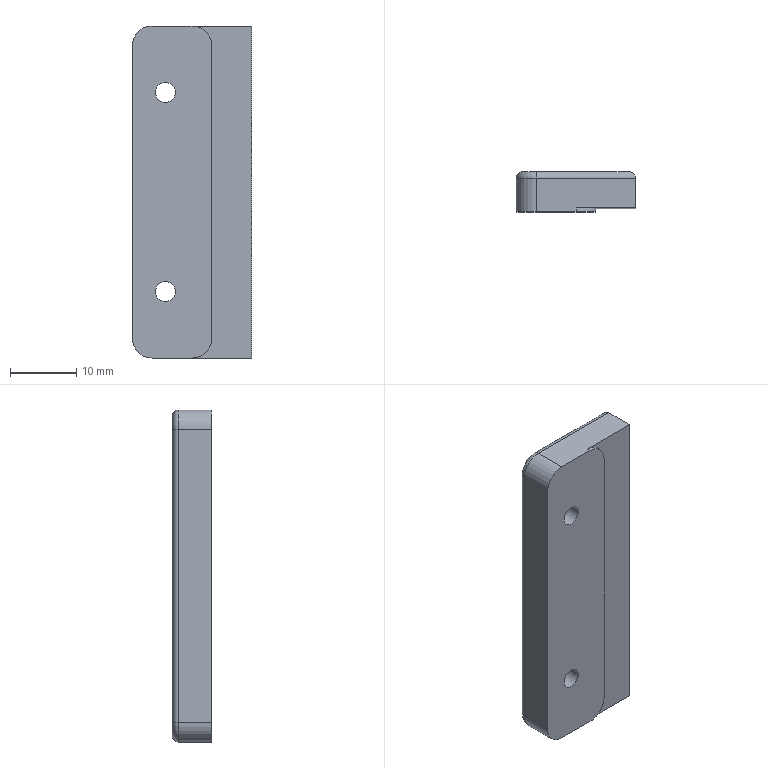Part | SolidWorks | features Fillet 4, ICE 3, Extrusion 1 | 1 solid | 28 faces | box 18 x 6 x 50 mm | volume 5021 mm3 | cylinder 16 | plane 10 | torus 2 | commonest cylinder face diameters 2 x4 3 x4 5 x4 6 x4
STEP:
#1=CARTESIAN_POINT('',(1.763,0.,10.));
#2=VERTEX_POINT('',#1);
#3=CARTESIAN_POINT('',(-1.237,0.,10.));
#4=VERTEX_POINT('',#3);
#5=CARTESIAN_POINT('',(0.2632,0.,10.));
#6=DIRECTION('',(0.,1.,0.));
#7=DIRECTION('',(-1.,0.,0.));
#8=AXIS2_PLACEMENT_3D('',#5,#6,#7);
#9=CIRCLE('',#8,1.5);
#10=EDGE_CURVE('',#2,#4,#9,.T.);
#11=ORIENTED_EDGE('',*,*,#10,.F.);
#12=CARTESIAN_POINT('',(1.763,3.,10.));
#13=VERTEX_POINT('',#12);
#14=CARTESIAN_POINT('',(1.763,0.,10.));
#15=DIRECTION('',(0.,1.,0.));
#16=VECTOR('',#15,1000.);
#17=LINE('',#14,#16);
#18=EDGE_CURVE('',#2,#13,#17,.T.);
#19=ORIENTED_EDGE('',*,*,#18,.T.);
#20=CARTESIAN_POINT('',(-1.237,3.,10.));
#21=VERTEX_POINT('',#20);
#22=CARTESIAN_POINT('',(0.2632,3.,10.));
#23=DIRECTION('',(0.,1.,0.));
#24=DIRECTION('',(-1.,0.,0.));
#25=AXIS2_PLACEMENT_3D('',#22,#23,#24);
#26=CIRCLE('',#25,1.5);
#27=EDGE_CURVE('',#13,#21,#26,.T.);
#28=ORIENTED_EDGE('',*,*,#27,.T.);
#29=CARTESIAN_POINT('',(-1.237,0.,10.));
#30=DIRECTION('',(0.,1.,0.));
#31=VECTOR('',#30,1000.);
#32=LINE('',#29,#31);
#33=EDGE_CURVE('',#4,#21,#32,.T.);
#34=ORIENTED_EDGE('',*,*,#33,.F.);
#35=EDGE_LOOP('',(#11,#19,#28,#34));
#36=FACE_OUTER_BOUND('',#35,.T.);
#37=CARTESIAN_POINT('',(0.2632,0.,10.));
#38=DIRECTION('',(0.,1.,0.));
#39=DIRECTION('',(-1.,0.,0.));
#40=AXIS2_PLACEMENT_3D('',#37,#38,#39);
#41=CYLINDRICAL_SURFACE('',#40,1.5);
#42=ADVANCED_FACE('',(#36),#41,.F.);
#43=CARTESIAN_POINT('',(1.763,0.,40.));
#44=VERTEX_POINT('',#43);
#45=CARTESIAN_POINT('',(-1.237,0.,40.));
#46=VERTEX_POINT('',#45);
#47=CARTESIAN_POINT('',(0.2632,0.,40.));
#48=DIRECTION('',(0.,1.,0.));
#49=DIRECTION('',(-1.,0.,0.));
#50=AXIS2_PLACEMENT_3D('',#47,#48,#49);
#51=CIRCLE('',#50,1.5);
#52=EDGE_CURVE('',#44,#46,#51,.T.);
#53=ORIENTED_EDGE('',*,*,#52,.F.);
#54=CARTESIAN_POINT('',(1.763,3.,40.));
#55=VERTEX_POINT('',#54);
#56=CARTESIAN_POINT('',(1.763,0.,40.));
#57=DIRECTION('',(0.,1.,0.));
#58=VECTOR('',#57,1000.);
#59=LINE('',#56,#58);
#60=EDGE_CURVE('',#44,#55,#59,.T.);
#61=ORIENTED_EDGE('',*,*,#60,.T.);
#62=CARTESIAN_POINT('',(-1.237,3.,40.));
#63=VERTEX_POINT('',#62);
#64=CARTESIAN_POINT('',(0.2632,3.,40.));
#65=DIRECTION('',(0.,1.,0.));
#66=DIRECTION('',(-1.,0.,0.));
#67=AXIS2_PLACEMENT_3D('',#64,#65,#66);
#68=CIRCLE('',#67,1.5);
#69=EDGE_CURVE('',#55,#63,#68,.T.);
#70=ORIENTED_EDGE('',*,*,#69,.T.);
#71=CARTESIAN_POINT('',(-1.237,0.,40.));
#72=DIRECTION('',(0.,1.,0.));
#73=VECTOR('',#72,1000.);
#74=LINE('',#71,#73);
#75=EDGE_CURVE('',#46,#63,#74,.T.);
#76=ORIENTED_EDGE('',*,*,#75,.F.);
#77=EDGE_LOOP('',(#53,#61,#70,#76));
#78=FACE_OUTER_BOUND('',#77,.T.);
#79=CARTESIAN_POINT('',(0.2632,0.,40.));
#80=DIRECTION('',(0.,1.,0.));
#81=DIRECTION('',(-1.,0.,0.));
#82=AXIS2_PLACEMENT_3D('',#79,#80,#81);
#83=CYLINDRICAL_SURFACE('',#82,1.5);
#84=ADVANCED_FACE('',(#78),#83,.F.);
#85=CARTESIAN_POINT('',(2.763,3.,10.));
#86=VERTEX_POINT('',#85);
#87=CARTESIAN_POINT('',(-2.237,3.,10.));
#88=VERTEX_POINT('',#87);
#89=CARTESIAN_POINT('',(0.2632,3.,10.));
#90=DIRECTION('',(0.,1.,0.));
#91=DIRECTION('',(-1.,0.,0.));
#92=AXIS2_PLACEMENT_3D('',#89,#90,#91);
#93=CIRCLE('',#92,2.5);
#94=EDGE_CURVE('',#86,#88,#93,.T.);
#95=ORIENTED_EDGE('',*,*,#94,.F.);
#96=CARTESIAN_POINT('',(2.763,6.,10.));
#97=VERTEX_POINT('',#96);
#98=CARTESIAN_POINT('',(2.763,3.,10.));
#99=DIRECTION('',(0.,1.,0.));
#100=VECTOR('',#99,1000.);
#101=LINE('',#98,#100);
#102=EDGE_CURVE('',#86,#97,#101,.T.);
#103=ORIENTED_EDGE('',*,*,#102,.T.);
#104=CARTESIAN_POINT('',(-2.237,6.,10.));
#105=VERTEX_POINT('',#104);
#106=CARTESIAN_POINT('',(0.2632,6.,10.));
#107=DIRECTION('',(0.,1.,0.));
#108=DIRECTION('',(-1.,0.,0.));
#109=AXIS2_PLACEMENT_3D('',#106,#107,#108);
#110=CIRCLE('',#109,2.5);
#111=EDGE_CURVE('',#97,#105,#110,.T.);
#112=ORIENTED_EDGE('',*,*,#111,.T.);
#113=CARTESIAN_POINT('',(-2.237,3.,10.));
#114=DIRECTION('',(0.,1.,0.));
#115=VECTOR('',#114,1000.);
#116=LINE('',#113,#115);
#117=EDGE_CURVE('',#88,#105,#116,.T.);
#118=ORIENTED_EDGE('',*,*,#117,.F.);
#119=EDGE_LOOP('',(#95,#103,#112,#118));
#120=FACE_OUTER_BOUND('',#119,.T.);
#121=CARTESIAN_POINT('',(0.2632,3.,10.));
#122=DIRECTION('',(0.,1.,0.));
#123=DIRECTION('',(-1.,0.,0.));
#124=AXIS2_PLACEMENT_3D('',#121,#122,#123);
#125=CYLINDRICAL_SURFACE('',#124,2.5);
#126=ADVANCED_FACE('',(#120),#125,.F.);
#127=CARTESIAN_POINT('',(2.763,3.,40.));
#128=VERTEX_POINT('',#127);
#129=CARTESIAN_POINT('',(-2.237,3.,40.));
#130=VERTEX_POINT('',#129);
#131=CARTESIAN_POINT('',(0.2632,3.,40.));
#132=DIRECTION('',(0.,1.,0.));
#133=DIRECTION('',(-1.,0.,0.));
#134=AXIS2_PLACEMENT_3D('',#131,#132,#133);
#135=CIRCLE('',#134,2.5);
#136=EDGE_CURVE('',#128,#130,#135,.T.);
#137=ORIENTED_EDGE('',*,*,#136,.F.);
#138=CARTESIAN_POINT('',(2.763,6.,40.));
#139=VERTEX_POINT('',#138);
#140=CARTESIAN_POINT('',(2.763,3.,40.));
#141=DIRECTION('',(0.,1.,0.));
#142=VECTOR('',#141,1000.);
#143=LINE('',#140,#142);
#144=EDGE_CURVE('',#128,#139,#143,.T.);
#145=ORIENTED_EDGE('',*,*,#144,.T.);
#146=CARTESIAN_POINT('',(-2.237,6.,40.));
#147=VERTEX_POINT('',#146);
#148=CARTESIAN_POINT('',(0.2632,6.,40.));
#149=DIRECTION('',(0.,1.,0.));
#150=DIRECTION('',(-1.,0.,0.));
#151=AXIS2_PLACEMENT_3D('',#148,#149,#150);
#152=CIRCLE('',#151,2.5);
#153=EDGE_CURVE('',#139,#147,#152,.T.);
#154=ORIENTED_EDGE('',*,*,#153,.T.);
#155=CARTESIAN_POINT('',(-2.237,3.,40.));
#156=DIRECTION('',(0.,1.,0.));
#157=VECTOR('',#156,1000.);
#158=LINE('',#155,#157);
#159=EDGE_CURVE('',#130,#147,#158,.T.);
#160=ORIENTED_EDGE('',*,*,#159,.F.);
#161=EDGE_LOOP('',(#137,#145,#154,#160));
#162=FACE_OUTER_BOUND('',#161,.T.);
#163=CARTESIAN_POINT('',(0.2632,3.,40.));
#164=DIRECTION('',(0.,1.,0.));
#165=DIRECTION('',(-1.,0.,0.));
#166=AXIS2_PLACEMENT_3D('',#163,#164,#165);
#167=CYLINDRICAL_SURFACE('',#166,2.5);
#168=ADVANCED_FACE('',(#162),#167,.F.);
#169=CARTESIAN_POINT('',(0.2632,0.,10.));
#170=DIRECTION('',(0.,1.,0.));
#171=DIRECTION('',(-1.,0.,0.));
#172=AXIS2_PLACEMENT_3D('',#169,#170,#171);
#173=CIRCLE('',#172,1.5);
#174=EDGE_CURVE('',#4,#2,#173,.T.);
#175=ORIENTED_EDGE('',*,*,#174,.T.);
#176=ORIENTED_EDGE('',*,*,#10,.T.);
#177=EDGE_LOOP('',(#175,#176));
#178=FACE_BOUND('',#177,.T.);
#179=CARTESIAN_POINT('',(0.2632,0.,40.));
#180=DIRECTION('',(0.,1.,0.));
#181=DIRECTION('',(-1.,0.,0.));
#182=AXIS2_PLACEMENT_3D('',#179,#180,#181);
#183=CIRCLE('',#182,1.5);
#184=EDGE_CURVE('',#46,#44,#183,.T.);
#185=ORIENTED_EDGE('',*,*,#184,.T.);
#186=ORIENTED_EDGE('',*,*,#52,.T.);
#187=EDGE_LOOP('',(#185,#186));
#188=FACE_BOUND('',#187,.T.);
#189=CARTESIAN_POINT('',(-4.737,0.,47.));
#190=VERTEX_POINT('',#189);
#191=CARTESIAN_POINT('',(-4.737,0.,3.));
#192=VERTEX_POINT('',#191);
#193=CARTESIAN_POINT('',(-4.737,0.,50.));
#194=DIRECTION('',(0.,0.,-1.));
#195=VECTOR('',#194,1000.);
#196=LINE('',#193,#195);
#197=EDGE_CURVE('',#190,#192,#196,.T.);
#198=ORIENTED_EDGE('',*,*,#197,.T.);
#199=CARTESIAN_POINT('',(-1.737,0.,0.));
#200=VERTEX_POINT('',#199);
#201=CARTESIAN_POINT('',(-1.737,0.,3.));
#202=DIRECTION('',(0.,-1.,0.));
#203=DIRECTION('',(-1.,0.,0.));
#204=AXIS2_PLACEMENT_3D('',#201,#202,#203);
#205=CIRCLE('',#204,3.);
#206=EDGE_CURVE('',#192,#200,#205,.T.);
#207=ORIENTED_EDGE('',*,*,#206,.T.);
#208=CARTESIAN_POINT('',(4.263,0.,0.));
#209=VERTEX_POINT('',#208);
#210=CARTESIAN_POINT('',(7.263,0.,0.));
#211=DIRECTION('',(1.,0.,0.));
#212=VECTOR('',#211,1000.);
#213=LINE('',#210,#212);
#214=EDGE_CURVE('',#200,#209,#213,.T.);
#215=ORIENTED_EDGE('',*,*,#214,.T.);
#216=CARTESIAN_POINT('',(7.263,0.,3.));
#217=VERTEX_POINT('',#216);
#218=CARTESIAN_POINT('',(4.263,0.,3.));
#219=DIRECTION('',(0.,-1.,0.));
#220=DIRECTION('',(-1.,0.,0.));
#221=AXIS2_PLACEMENT_3D('',#218,#219,#220);
#222=CIRCLE('',#221,3.);
#223=EDGE_CURVE('',#209,#217,#222,.T.);
#224=ORIENTED_EDGE('',*,*,#223,.T.);
#225=CARTESIAN_POINT('',(7.263,0.,47.));
#226=VERTEX_POINT('',#225);
#227=CARTESIAN_POINT('',(7.263,0.,50.));
#228=DIRECTION('',(0.,0.,-1.));
#229=VECTOR('',#228,1000.);
#230=LINE('',#227,#229);
#231=EDGE_CURVE('',#226,#217,#230,.T.);
#232=ORIENTED_EDGE('',*,*,#231,.F.);
#233=CARTESIAN_POINT('',(4.263,0.,50.));
#234=VERTEX_POINT('',#233);
#235=CARTESIAN_POINT('',(4.263,0.,47.));
#236=DIRECTION('',(0.,-1.,0.));
#237=DIRECTION('',(-1.,0.,0.));
#238=AXIS2_PLACEMENT_3D('',#235,#236,#237);
#239=CIRCLE('',#238,3.);
#240=EDGE_CURVE('',#226,#234,#239,.T.);
#241=ORIENTED_EDGE('',*,*,#240,.T.);
#242=CARTESIAN_POINT('',(-1.737,0.,50.));
#243=VERTEX_POINT('',#242);
#244=CARTESIAN_POINT('',(7.263,0.,50.));
#245=DIRECTION('',(1.,0.,0.));
#246=VECTOR('',#245,1000.);
#247=LINE('',#244,#246);
#248=EDGE_CURVE('',#243,#234,#247,.T.);
#249=ORIENTED_EDGE('',*,*,#248,.F.);
#250=CARTESIAN_POINT('',(-1.737,0.,47.));
#251=DIRECTION('',(0.,-1.,0.));
#252=DIRECTION('',(-1.,0.,0.));
#253=AXIS2_PLACEMENT_3D('',#250,#251,#252);
#254=CIRCLE('',#253,3.);
#255=EDGE_CURVE('',#243,#190,#254,.T.);
#256=ORIENTED_EDGE('',*,*,#255,.T.);
#257=EDGE_LOOP('',(#198,#207,#215,#224,#232,#241,#249,#256));
#258=FACE_OUTER_BOUND('',#257,.T.);
#259=CARTESIAN_POINT('',(7.263,0.,50.));
#260=DIRECTION('',(0.,1.,0.));
#261=DIRECTION('',(-1.,0.,0.));
#262=AXIS2_PLACEMENT_3D('',#259,#260,#261);
#263=PLANE('',#262);
#264=ADVANCED_FACE('',(#178,#188,#258),#263,.F.);
#265=ORIENTED_EDGE('',*,*,#231,.T.);
#266=CARTESIAN_POINT('',(7.263,0.55,3.));
#267=VERTEX_POINT('',#266);
#268=CARTESIAN_POINT('',(7.263,0.55,3.));
#269=DIRECTION('',(0.,1.,0.));
#270=VECTOR('',#269,1000.);
#271=LINE('',#268,#270);
#272=EDGE_CURVE('',#217,#267,#271,.T.);
#273=ORIENTED_EDGE('',*,*,#272,.T.);
#274=CARTESIAN_POINT('',(7.263,0.55,47.));
#275=VERTEX_POINT('',#274);
#276=CARTESIAN_POINT('',(7.263,0.55,50.));
#277=DIRECTION('',(0.,0.,-1.));
#278=VECTOR('',#277,1000.);
#279=LINE('',#276,#278);
#280=EDGE_CURVE('',#275,#267,#279,.T.);
#281=ORIENTED_EDGE('',*,*,#280,.F.);
#282=CARTESIAN_POINT('',(7.263,0.55,47.));
#283=DIRECTION('',(0.,-1.,0.));
#284=VECTOR('',#283,1000.);
#285=LINE('',#282,#284);
#286=EDGE_CURVE('',#275,#226,#285,.T.);
#287=ORIENTED_EDGE('',*,*,#286,.T.);
#288=EDGE_LOOP('',(#265,#273,#281,#287));
#289=FACE_OUTER_BOUND('',#288,.T.);
#290=CARTESIAN_POINT('',(7.263,0.55,50.));
#291=DIRECTION('',(-1.,0.,0.));
#292=DIRECTION('',(0.,-1.,0.));
#293=AXIS2_PLACEMENT_3D('',#290,#291,#292);
#294=PLANE('',#293);
#295=ADVANCED_FACE('',(#289),#294,.F.);
#296=CARTESIAN_POINT('',(4.263,0.55,0.));
#297=VERTEX_POINT('',#296);
#298=CARTESIAN_POINT('',(13.263,0.55,0.));
#299=VERTEX_POINT('',#298);
#300=CARTESIAN_POINT('',(13.263,0.55,0.));
#301=DIRECTION('',(1.,0.,0.));
#302=VECTOR('',#301,1000.);
#303=LINE('',#300,#302);
#304=EDGE_CURVE('',#297,#299,#303,.T.);
#305=ORIENTED_EDGE('',*,*,#304,.T.);
#306=CARTESIAN_POINT('',(13.263,0.55,50.));
#307=VERTEX_POINT('',#306);
#308=CARTESIAN_POINT('',(13.263,0.55,50.));
#309=DIRECTION('',(0.,0.,-1.));
#310=VECTOR('',#309,1000.);
#311=LINE('',#308,#310);
#312=EDGE_CURVE('',#307,#299,#311,.T.);
#313=ORIENTED_EDGE('',*,*,#312,.F.);
#314=CARTESIAN_POINT('',(4.263,0.55,50.));
#315=VERTEX_POINT('',#314);
#316=CARTESIAN_POINT('',(13.263,0.55,50.));
#317=DIRECTION('',(1.,0.,0.));
#318=VECTOR('',#317,1000.);
#319=LINE('',#316,#318);
#320=EDGE_CURVE('',#315,#307,#319,.T.);
#321=ORIENTED_EDGE('',*,*,#320,.F.);
#322=CARTESIAN_POINT('',(4.263,0.55,47.));
#323=DIRECTION('',(0.,1.,0.));
#324=DIRECTION('',(-1.,0.,0.));
#325=AXIS2_PLACEMENT_3D('',#322,#323,#324);
#326=CIRCLE('',#325,3.);
#327=EDGE_CURVE('',#315,#275,#326,.T.);
#328=ORIENTED_EDGE('',*,*,#327,.T.);
#329=ORIENTED_EDGE('',*,*,#280,.T.);
#330=CARTESIAN_POINT('',(4.263,0.55,3.));
#331=DIRECTION('',(0.,1.,0.));
#332=DIRECTION('',(-1.,0.,0.));
#333=AXIS2_PLACEMENT_3D('',#330,#331,#332);
#334=CIRCLE('',#333,3.);
#335=EDGE_CURVE('',#267,#297,#334,.T.);
#336=ORIENTED_EDGE('',*,*,#335,.T.);
#337=EDGE_LOOP('',(#305,#313,#321,#328,#329,#336));
#338=FACE_OUTER_BOUND('',#337,.T.);
#339=CARTESIAN_POINT('',(13.263,0.55,50.));
#340=DIRECTION('',(0.,1.,0.));
#341=DIRECTION('',(-1.,0.,0.));
#342=AXIS2_PLACEMENT_3D('',#339,#340,#341);
#343=PLANE('',#342);
#344=ADVANCED_FACE('',(#338),#343,.F.);
#345=CARTESIAN_POINT('',(13.263,5.,0.));
#346=VERTEX_POINT('',#345);
#347=CARTESIAN_POINT('',(13.263,6.,0.));
#348=DIRECTION('',(0.,1.,0.));
#349=VECTOR('',#348,1000.);
#350=LINE('',#347,#349);
#351=EDGE_CURVE('',#299,#346,#350,.T.);
#352=ORIENTED_EDGE('',*,*,#351,.T.);
#353=CARTESIAN_POINT('',(13.263,5.,50.));
#354=VERTEX_POINT('',#353);
#355=CARTESIAN_POINT('',(13.263,5.,50.));
#356=DIRECTION('',(0.,0.,1.));
#357=VECTOR('',#356,1000.);
#358=LINE('',#355,#357);
#359=EDGE_CURVE('',#346,#354,#358,.T.);
#360=ORIENTED_EDGE('',*,*,#359,.T.);
#361=CARTESIAN_POINT('',(13.263,6.,50.));
#362=DIRECTION('',(0.,1.,0.));
#363=VECTOR('',#362,1000.);
#364=LINE('',#361,#363);
#365=EDGE_CURVE('',#307,#354,#364,.T.);
#366=ORIENTED_EDGE('',*,*,#365,.F.);
#367=ORIENTED_EDGE('',*,*,#312,.T.);
#368=EDGE_LOOP('',(#352,#360,#366,#367));
#369=FACE_OUTER_BOUND('',#368,.T.);
#370=CARTESIAN_POINT('',(13.263,6.,50.));
#371=DIRECTION('',(-1.,0.,0.));
#372=DIRECTION('',(0.,0.,1.));
#373=AXIS2_PLACEMENT_3D('',#370,#371,#372);
#374=PLANE('',#373);
#375=ADVANCED_FACE('',(#369),#374,.F.);
#376=CARTESIAN_POINT('',(-3.737,6.,47.));
#377=VERTEX_POINT('',#376);
#378=CARTESIAN_POINT('',(-1.737,6.,49.));
#379=VERTEX_POINT('',#378);
#380=CARTESIAN_POINT('',(-1.737,6.,47.));
#381=DIRECTION('',(0.,1.,0.));
#382=DIRECTION('',(0.,0.,-1.));
#383=AXIS2_PLACEMENT_3D('',#380,#381,#382);
#384=CIRCLE('',#383,2.);
#385=EDGE_CURVE('',#377,#379,#384,.T.);
#386=ORIENTED_EDGE('',*,*,#385,.T.);
#387=CARTESIAN_POINT('',(12.263,6.,49.));
#388=VERTEX_POINT('',#387);
#389=CARTESIAN_POINT('',(-4.737,6.,49.));
#390=DIRECTION('',(1.,0.,0.));
#391=VECTOR('',#390,1000.);
#392=LINE('',#389,#391);
#393=EDGE_CURVE('',#379,#388,#392,.T.);
#394=ORIENTED_EDGE('',*,*,#393,.T.);
#395=CARTESIAN_POINT('',(12.263,6.,1.));
#396=VERTEX_POINT('',#395);
#397=CARTESIAN_POINT('',(12.263,6.,50.));
#398=DIRECTION('',(0.,0.,-1.));
#399=VECTOR('',#398,1000.);
#400=LINE('',#397,#399);
#401=EDGE_CURVE('',#388,#396,#400,.T.);
#402=ORIENTED_EDGE('',*,*,#401,.T.);
#403=CARTESIAN_POINT('',(-1.737,6.,1.));
#404=VERTEX_POINT('',#403);
#405=CARTESIAN_POINT('',(-1.737,6.,1.));
#406=DIRECTION('',(-1.,0.,0.));
#407=VECTOR('',#406,1000.);
#408=LINE('',#405,#407);
#409=EDGE_CURVE('',#396,#404,#408,.T.);
#410=ORIENTED_EDGE('',*,*,#409,.T.);
#411=CARTESIAN_POINT('',(-3.737,6.,3.));
#412=VERTEX_POINT('',#411);
#413=CARTESIAN_POINT('',(-1.737,6.,3.));
#414=DIRECTION('',(0.,1.,0.));
#415=DIRECTION('',(0.,0.,-1.));
#416=AXIS2_PLACEMENT_3D('',#413,#414,#415);
#417=CIRCLE('',#416,2.);
#418=EDGE_CURVE('',#404,#412,#417,.T.);
#419=ORIENTED_EDGE('',*,*,#418,.T.);
#420=CARTESIAN_POINT('',(-3.737,6.,50.));
#421=DIRECTION('',(0.,0.,1.));
#422=VECTOR('',#421,1000.);
#423=LINE('',#420,#422);
#424=EDGE_CURVE('',#412,#377,#423,.T.);
#425=ORIENTED_EDGE('',*,*,#424,.T.);
#426=EDGE_LOOP('',(#386,#394,#402,#410,#419,#425));
#427=FACE_OUTER_BOUND('',#426,.T.);
#428=CARTESIAN_POINT('',(0.2632,6.,10.));
#429=DIRECTION('',(0.,1.,0.));
#430=DIRECTION('',(-1.,0.,0.));
#431=AXIS2_PLACEMENT_3D('',#428,#429,#430);
#432=CIRCLE('',#431,2.5);
#433=EDGE_CURVE('',#105,#97,#432,.T.);
#434=ORIENTED_EDGE('',*,*,#433,.F.);
#435=ORIENTED_EDGE('',*,*,#111,.F.);
#436=EDGE_LOOP('',(#434,#435));
#437=FACE_BOUND('',#436,.T.);
#438=CARTESIAN_POINT('',(0.2632,6.,40.));
#439=DIRECTION('',(0.,1.,0.));
#440=DIRECTION('',(-1.,0.,0.));
#441=AXIS2_PLACEMENT_3D('',#438,#439,#440);
#442=CIRCLE('',#441,2.5);
#443=EDGE_CURVE('',#147,#139,#442,.T.);
#444=ORIENTED_EDGE('',*,*,#443,.F.);
#445=ORIENTED_EDGE('',*,*,#153,.F.);
#446=EDGE_LOOP('',(#444,#445));
#447=FACE_BOUND('',#446,.T.);
#448=CARTESIAN_POINT('',(-4.737,6.,50.));
#449=DIRECTION('',(0.,-1.,0.));
#450=DIRECTION('',(0.,0.,-1.));
#451=AXIS2_PLACEMENT_3D('',#448,#449,#450);
#452=PLANE('',#451);
#453=ADVANCED_FACE('',(#427,#437,#447),#452,.F.);
#454=CARTESIAN_POINT('',(-4.737,5.,47.));
#455=VERTEX_POINT('',#454);
#456=CARTESIAN_POINT('',(-4.737,0.,47.));
#457=DIRECTION('',(0.,1.,0.));
#458=VECTOR('',#457,1000.);
#459=LINE('',#456,#458);
#460=EDGE_CURVE('',#190,#455,#459,.T.);
#461=ORIENTED_EDGE('',*,*,#460,.T.);
#462=CARTESIAN_POINT('',(-4.737,5.,3.));
#463=VERTEX_POINT('',#462);
#464=CARTESIAN_POINT('',(-4.737,5.,50.));
#465=DIRECTION('',(0.,0.,-1.));
#466=VECTOR('',#465,1000.);
#467=LINE('',#464,#466);
#468=EDGE_CURVE('',#455,#463,#467,.T.);
#469=ORIENTED_EDGE('',*,*,#468,.T.);
#470=CARTESIAN_POINT('',(-4.737,0.,3.));
#471=DIRECTION('',(0.,-1.,0.));
#472=VECTOR('',#471,1000.);
#473=LINE('',#470,#472);
#474=EDGE_CURVE('',#463,#192,#473,.T.);
#475=ORIENTED_EDGE('',*,*,#474,.T.);
#476=ORIENTED_EDGE('',*,*,#197,.F.);
#477=EDGE_LOOP('',(#461,#469,#475,#476));
#478=FACE_OUTER_BOUND('',#477,.T.);
#479=CARTESIAN_POINT('',(-4.737,0.,50.));
#480=DIRECTION('',(1.,0.,0.));
#481=DIRECTION('',(0.,0.,-1.));
#482=AXIS2_PLACEMENT_3D('',#479,#480,#481);
#483=PLANE('',#482);
#484=ADVANCED_FACE('',(#478),#483,.F.);
#485=ORIENTED_EDGE('',*,*,#365,.T.);
#486=CARTESIAN_POINT('',(-1.737,5.,50.));
#487=VERTEX_POINT('',#486);
#488=CARTESIAN_POINT('',(0.,5.,50.));
#489=DIRECTION('',(-1.,0.,0.));
#490=VECTOR('',#489,1000.);
#491=LINE('',#488,#490);
#492=EDGE_CURVE('',#354,#487,#491,.T.);
#493=ORIENTED_EDGE('',*,*,#492,.T.);
#494=CARTESIAN_POINT('',(-1.737,0.,50.));
#495=DIRECTION('',(0.,-1.,0.));
#496=VECTOR('',#495,1000.);
#497=LINE('',#494,#496);
#498=EDGE_CURVE('',#487,#243,#497,.T.);
#499=ORIENTED_EDGE('',*,*,#498,.T.);
#500=ORIENTED_EDGE('',*,*,#248,.T.);
#501=CARTESIAN_POINT('',(4.263,0.,50.));
#502=DIRECTION('',(0.,1.,0.));
#503=VECTOR('',#502,1000.);
#504=LINE('',#501,#503);
#505=EDGE_CURVE('',#234,#315,#504,.T.);
#506=ORIENTED_EDGE('',*,*,#505,.T.);
#507=ORIENTED_EDGE('',*,*,#320,.T.);
#508=EDGE_LOOP('',(#485,#493,#499,#500,#506,#507));
#509=FACE_OUTER_BOUND('',#508,.T.);
#510=CARTESIAN_POINT('',(0.,0.,50.));
#511=DIRECTION('',(0.,0.,-1.));
#512=DIRECTION('',(-1.,0.,0.));
#513=AXIS2_PLACEMENT_3D('',#510,#511,#512);
#514=PLANE('',#513);
#515=ADVANCED_FACE('',(#509),#514,.F.);
#516=CARTESIAN_POINT('',(-1.737,5.,0.));
#517=VERTEX_POINT('',#516);
#518=CARTESIAN_POINT('',(-1.737,6.,0.));
#519=DIRECTION('',(0.,1.,0.));
#520=VECTOR('',#519,1000.);
#521=LINE('',#518,#520);
#522=EDGE_CURVE('',#200,#517,#521,.T.);
#523=ORIENTED_EDGE('',*,*,#522,.T.);
#524=CARTESIAN_POINT('',(13.263,5.,0.));
#525=DIRECTION('',(1.,0.,0.));
#526=VECTOR('',#525,1000.);
#527=LINE('',#524,#526);
#528=EDGE_CURVE('',#517,#346,#527,.T.);
#529=ORIENTED_EDGE('',*,*,#528,.T.);
#530=ORIENTED_EDGE('',*,*,#351,.F.);
#531=ORIENTED_EDGE('',*,*,#304,.F.);
#532=CARTESIAN_POINT('',(4.263,0.,0.));
#533=DIRECTION('',(0.,-1.,0.));
#534=VECTOR('',#533,1000.);
#535=LINE('',#532,#534);
#536=EDGE_CURVE('',#297,#209,#535,.T.);
#537=ORIENTED_EDGE('',*,*,#536,.T.);
#538=ORIENTED_EDGE('',*,*,#214,.F.);
#539=EDGE_LOOP('',(#523,#529,#530,#531,#537,#538));
#540=FACE_OUTER_BOUND('',#539,.T.);
#541=CARTESIAN_POINT('',(0.,0.,0.));
#542=DIRECTION('',(0.,0.,-1.));
#543=DIRECTION('',(-1.,0.,0.));
#544=AXIS2_PLACEMENT_3D('',#541,#542,#543);
#545=PLANE('',#544);
#546=ADVANCED_FACE('',(#540),#545,.T.);
#547=ORIENTED_EDGE('',*,*,#240,.F.);
#548=ORIENTED_EDGE('',*,*,#286,.F.);
#549=ORIENTED_EDGE('',*,*,#327,.F.);
#550=ORIENTED_EDGE('',*,*,#505,.F.);
#551=EDGE_LOOP('',(#547,#548,#549,#550));
#552=FACE_OUTER_BOUND('',#551,.T.);
#553=CARTESIAN_POINT('',(4.263,0.,47.));
#554=DIRECTION('',(0.,1.,0.));
#555=DIRECTION('',(-1.,0.,0.));
#556=AXIS2_PLACEMENT_3D('',#553,#554,#555);
#557=CYLINDRICAL_SURFACE('',#556,3.);
#558=ADVANCED_FACE('',(#552),#557,.T.);
#559=ORIENTED_EDGE('',*,*,#144,.F.);
#560=CARTESIAN_POINT('',(0.2632,3.,40.));
#561=DIRECTION('',(0.,1.,0.));
#562=DIRECTION('',(-1.,0.,0.));
#563=AXIS2_PLACEMENT_3D('',#560,#561,#562);
#564=CIRCLE('',#563,2.5);
#565=EDGE_CURVE('',#130,#128,#564,.T.);
#566=ORIENTED_EDGE('',*,*,#565,.F.);
#567=ORIENTED_EDGE('',*,*,#159,.T.);
#568=ORIENTED_EDGE('',*,*,#443,.T.);
#569=EDGE_LOOP('',(#559,#566,#567,#568));
#570=FACE_OUTER_BOUND('',#569,.T.);
#571=CARTESIAN_POINT('',(0.2632,3.,40.));
#572=DIRECTION('',(0.,1.,0.));
#573=DIRECTION('',(-1.,0.,0.));
#574=AXIS2_PLACEMENT_3D('',#571,#572,#573);
#575=CYLINDRICAL_SURFACE('',#574,2.5);
#576=ADVANCED_FACE('',(#570),#575,.F.);
#577=CARTESIAN_POINT('',(0.2632,3.,40.));
#578=DIRECTION('',(0.,1.,0.));
#579=DIRECTION('',(-1.,0.,0.));
#580=AXIS2_PLACEMENT_3D('',#577,#578,#579);
#581=CIRCLE('',#580,1.5);
#582=EDGE_CURVE('',#63,#55,#581,.T.);
#583=ORIENTED_EDGE('',*,*,#582,.F.);
#584=ORIENTED_EDGE('',*,*,#69,.F.);
#585=EDGE_LOOP('',(#583,#584));
#586=FACE_BOUND('',#585,.T.);
#587=ORIENTED_EDGE('',*,*,#565,.T.);
#588=ORIENTED_EDGE('',*,*,#136,.T.);
#589=EDGE_LOOP('',(#587,#588));
#590=FACE_OUTER_BOUND('',#589,.T.);
#591=CARTESIAN_POINT('',(0.2632,3.,40.));
#592=DIRECTION('',(0.,1.,0.));
#593=DIRECTION('',(-1.,0.,0.));
#594=AXIS2_PLACEMENT_3D('',#591,#592,#593);
#595=PLANE('',#594);
#596=ADVANCED_FACE('',(#586,#590),#595,.T.);
#597=ORIENTED_EDGE('',*,*,#102,.F.);
#598=CARTESIAN_POINT('',(0.2632,3.,10.));
#599=DIRECTION('',(0.,1.,0.));
#600=DIRECTION('',(-1.,0.,0.));
#601=AXIS2_PLACEMENT_3D('',#598,#599,#600);
#602=CIRCLE('',#601,2.5);
#603=EDGE_CURVE('',#88,#86,#602,.T.);
#604=ORIENTED_EDGE('',*,*,#603,.F.);
#605=ORIENTED_EDGE('',*,*,#117,.T.);
#606=ORIENTED_EDGE('',*,*,#433,.T.);
#607=EDGE_LOOP('',(#597,#604,#605,#606));
#608=FACE_OUTER_BOUND('',#607,.T.);
#609=CARTESIAN_POINT('',(0.2632,3.,10.));
#610=DIRECTION('',(0.,1.,0.));
#611=DIRECTION('',(-1.,0.,0.));
#612=AXIS2_PLACEMENT_3D('',#609,#610,#611);
#613=CYLINDRICAL_SURFACE('',#612,2.5);
#614=ADVANCED_FACE('',(#608),#613,.F.);
#615=CARTESIAN_POINT('',(0.2632,3.,10.));
#616=DIRECTION('',(0.,1.,0.));
#617=DIRECTION('',(-1.,0.,0.));
#618=AXIS2_PLACEMENT_3D('',#615,#616,#617);
#619=CIRCLE('',#618,1.5);
#620=EDGE_CURVE('',#21,#13,#619,.T.);
#621=ORIENTED_EDGE('',*,*,#620,.F.);
#622=ORIENTED_EDGE('',*,*,#27,.F.);
#623=EDGE_LOOP('',(#621,#622));
#624=FACE_BOUND('',#623,.T.);
#625=ORIENTED_EDGE('',*,*,#603,.T.);
#626=ORIENTED_EDGE('',*,*,#94,.T.);
#627=EDGE_LOOP('',(#625,#626));
#628=FACE_OUTER_BOUND('',#627,.T.);
#629=CARTESIAN_POINT('',(0.2632,3.,10.));
#630=DIRECTION('',(0.,1.,0.));
#631=DIRECTION('',(-1.,0.,0.));
#632=AXIS2_PLACEMENT_3D('',#629,#630,#631);
#633=PLANE('',#632);
#634=ADVANCED_FACE('',(#624,#628),#633,.T.);
#635=ORIENTED_EDGE('',*,*,#60,.F.);
#636=ORIENTED_EDGE('',*,*,#184,.F.);
#637=ORIENTED_EDGE('',*,*,#75,.T.);
#638=ORIENTED_EDGE('',*,*,#582,.T.);
#639=EDGE_LOOP('',(#635,#636,#637,#638));
#640=FACE_OUTER_BOUND('',#639,.T.);
#641=CARTESIAN_POINT('',(0.2632,0.,40.));
#642=DIRECTION('',(0.,1.,0.));
#643=DIRECTION('',(-1.,0.,0.));
#644=AXIS2_PLACEMENT_3D('',#641,#642,#643);
#645=CYLINDRICAL_SURFACE('',#644,1.5);
#646=ADVANCED_FACE('',(#640),#645,.F.);
#647=ORIENTED_EDGE('',*,*,#18,.F.);
#648=ORIENTED_EDGE('',*,*,#174,.F.);
#649=ORIENTED_EDGE('',*,*,#33,.T.);
#650=ORIENTED_EDGE('',*,*,#620,.T.);
#651=EDGE_LOOP('',(#647,#648,#649,#650));
#652=FACE_OUTER_BOUND('',#651,.T.);
#653=CARTESIAN_POINT('',(0.2632,0.,10.));
#654=DIRECTION('',(0.,1.,0.));
#655=DIRECTION('',(-1.,0.,0.));
#656=AXIS2_PLACEMENT_3D('',#653,#654,#655);
#657=CYLINDRICAL_SURFACE('',#656,1.5);
#658=ADVANCED_FACE('',(#652),#657,.F.);
#659=ORIENTED_EDGE('',*,*,#223,.F.);
#660=ORIENTED_EDGE('',*,*,#536,.F.);
#661=ORIENTED_EDGE('',*,*,#335,.F.);
#662=ORIENTED_EDGE('',*,*,#272,.F.);
#663=EDGE_LOOP('',(#659,#660,#661,#662));
#664=FACE_OUTER_BOUND('',#663,.T.);
#665=CARTESIAN_POINT('',(4.263,0.55,3.));
#666=DIRECTION('',(0.,-1.,0.));
#667=DIRECTION('',(1.,0.,0.));
#668=AXIS2_PLACEMENT_3D('',#665,#666,#667);
#669=CYLINDRICAL_SURFACE('',#668,3.);
#670=ADVANCED_FACE('',(#664),#669,.T.);
#671=ORIENTED_EDGE('',*,*,#474,.F.);
#672=CARTESIAN_POINT('',(-1.737,5.,3.));
#673=DIRECTION('',(0.,-1.,0.));
#674=DIRECTION('',(0.,0.,-1.));
#675=AXIS2_PLACEMENT_3D('',#672,#673,#674);
#676=CIRCLE('',#675,3.);
#677=EDGE_CURVE('',#463,#517,#676,.T.);
#678=ORIENTED_EDGE('',*,*,#677,.T.);
#679=ORIENTED_EDGE('',*,*,#522,.F.);
#680=ORIENTED_EDGE('',*,*,#206,.F.);
#681=EDGE_LOOP('',(#671,#678,#679,#680));
#682=FACE_OUTER_BOUND('',#681,.T.);
#683=CARTESIAN_POINT('',(-1.737,0.,3.));
#684=DIRECTION('',(0.,1.,0.));
#685=DIRECTION('',(0.,0.,1.));
#686=AXIS2_PLACEMENT_3D('',#683,#684,#685);
#687=CYLINDRICAL_SURFACE('',#686,3.);
#688=ADVANCED_FACE('',(#682),#687,.T.);
#689=ORIENTED_EDGE('',*,*,#498,.F.);
#690=CARTESIAN_POINT('',(-1.737,5.,47.));
#691=DIRECTION('',(0.,-1.,0.));
#692=DIRECTION('',(0.,0.,-1.));
#693=AXIS2_PLACEMENT_3D('',#690,#691,#692);
#694=CIRCLE('',#693,3.);
#695=EDGE_CURVE('',#487,#455,#694,.T.);
#696=ORIENTED_EDGE('',*,*,#695,.T.);
#697=ORIENTED_EDGE('',*,*,#460,.F.);
#698=ORIENTED_EDGE('',*,*,#255,.F.);
#699=EDGE_LOOP('',(#689,#696,#697,#698));
#700=FACE_OUTER_BOUND('',#699,.T.);
#701=CARTESIAN_POINT('',(-1.737,0.,47.));
#702=DIRECTION('',(0.,-1.,0.));
#703=DIRECTION('',(0.,0.,-1.));
#704=AXIS2_PLACEMENT_3D('',#701,#702,#703);
#705=CYLINDRICAL_SURFACE('',#704,3.);
#706=ADVANCED_FACE('',(#700),#705,.T.);
#707=CARTESIAN_POINT('',(-3.737,5.,3.));
#708=DIRECTION('',(0.,0.,1.));
#709=DIRECTION('',(1.,0.,0.));
#710=AXIS2_PLACEMENT_3D('',#707,#708,#709);
#711=CIRCLE('',#710,1.);
#712=EDGE_CURVE('',#412,#463,#711,.T.);
#713=ORIENTED_EDGE('',*,*,#712,.F.);
#714=ORIENTED_EDGE('',*,*,#418,.F.);
#715=CARTESIAN_POINT('',(-1.737,5.,1.));
#716=DIRECTION('',(1.,0.,0.));
#717=DIRECTION('',(0.,0.,-1.));
#718=AXIS2_PLACEMENT_3D('',#715,#716,#717);
#719=CIRCLE('',#718,1.);
#720=EDGE_CURVE('',#517,#404,#719,.T.);
#721=ORIENTED_EDGE('',*,*,#720,.F.);
#722=ORIENTED_EDGE('',*,*,#677,.F.);
#723=EDGE_LOOP('',(#713,#714,#721,#722));
#724=FACE_OUTER_BOUND('',#723,.T.);
#725=CARTESIAN_POINT('',(-1.737,5.,3.));
#726=DIRECTION('',(0.,-1.,0.));
#727=DIRECTION('',(0.,0.,-1.));
#728=AXIS2_PLACEMENT_3D('',#725,#726,#727);
#729=TOROIDAL_SURFACE('',#728,2.,1.);
#730=ADVANCED_FACE('',(#724),#729,.T.);
#731=ORIENTED_EDGE('',*,*,#720,.T.);
#732=ORIENTED_EDGE('',*,*,#409,.F.);
#733=CARTESIAN_POINT('',(13.263,5.,0.));
#734=CARTESIAN_POINT('',(13.263,5.586,0.));
#735=CARTESIAN_POINT('',(12.849,6.,0.4142));
#736=CARTESIAN_POINT('',(12.263,6.,1.));
#737=(BOUNDED_CURVE()B_SPLINE_CURVE(3,(#733,#734,#735,#736),.UNSPECIFIED.,.F.,.F.)B_SPLINE_CURVE_WITH_KNOTS((4,4),(0.,1.571),.UNSPECIFIED.)CURVE()GEOMETRIC_REPRESENTATION_ITEM()RATIONAL_B_SPLINE_CURVE((1.,0.8047,0.8047,1.))REPRESENTATION_ITEM(''));
#738=EDGE_CURVE('',#346,#396,#737,.T.);
#739=ORIENTED_EDGE('',*,*,#738,.F.);
#740=ORIENTED_EDGE('',*,*,#528,.F.);
#741=EDGE_LOOP('',(#731,#732,#739,#740));
#742=FACE_OUTER_BOUND('',#741,.T.);
#743=CARTESIAN_POINT('',(-4.737,5.,1.));
#744=DIRECTION('',(1.,0.,0.));
#745=DIRECTION('',(0.,0.,-1.));
#746=AXIS2_PLACEMENT_3D('',#743,#744,#745);
#747=CYLINDRICAL_SURFACE('',#746,1.);
#748=ADVANCED_FACE('',(#742),#747,.T.);
#749=ORIENTED_EDGE('',*,*,#712,.T.);
#750=ORIENTED_EDGE('',*,*,#468,.F.);
#751=CARTESIAN_POINT('',(-3.737,5.,47.));
#752=DIRECTION('',(0.,0.,1.));
#753=DIRECTION('',(1.,0.,0.));
#754=AXIS2_PLACEMENT_3D('',#751,#752,#753);
#755=CIRCLE('',#754,1.);
#756=EDGE_CURVE('',#377,#455,#755,.T.);
#757=ORIENTED_EDGE('',*,*,#756,.F.);
#758=ORIENTED_EDGE('',*,*,#424,.F.);
#759=EDGE_LOOP('',(#749,#750,#757,#758));
#760=FACE_OUTER_BOUND('',#759,.T.);
#761=CARTESIAN_POINT('',(-3.737,5.,50.));
#762=DIRECTION('',(0.,0.,-1.));
#763=DIRECTION('',(-1.,0.,0.));
#764=AXIS2_PLACEMENT_3D('',#761,#762,#763);
#765=CYLINDRICAL_SURFACE('',#764,1.);
#766=ADVANCED_FACE('',(#760),#765,.T.);
#767=ORIENTED_EDGE('',*,*,#738,.T.);
#768=ORIENTED_EDGE('',*,*,#401,.F.);
#769=CARTESIAN_POINT('',(13.263,5.,50.));
#770=CARTESIAN_POINT('',(13.263,5.586,50.));
#771=CARTESIAN_POINT('',(12.849,6.,49.586));
#772=CARTESIAN_POINT('',(12.263,6.,49.));
#773=(BOUNDED_CURVE()B_SPLINE_CURVE(3,(#769,#770,#771,#772),.UNSPECIFIED.,.F.,.F.)B_SPLINE_CURVE_WITH_KNOTS((4,4),(3.142,4.712),.UNSPECIFIED.)CURVE()GEOMETRIC_REPRESENTATION_ITEM()RATIONAL_B_SPLINE_CURVE((1.,0.8047,0.8047,1.))REPRESENTATION_ITEM(''));
#774=EDGE_CURVE('',#354,#388,#773,.T.);
#775=ORIENTED_EDGE('',*,*,#774,.F.);
#776=ORIENTED_EDGE('',*,*,#359,.F.);
#777=EDGE_LOOP('',(#767,#768,#775,#776));
#778=FACE_OUTER_BOUND('',#777,.T.);
#779=CARTESIAN_POINT('',(12.263,5.,50.));
#780=DIRECTION('',(0.,0.,-1.));
#781=DIRECTION('',(-1.,0.,0.));
#782=AXIS2_PLACEMENT_3D('',#779,#780,#781);
#783=CYLINDRICAL_SURFACE('',#782,1.);
#784=ADVANCED_FACE('',(#778),#783,.T.);
#785=ORIENTED_EDGE('',*,*,#756,.T.);
#786=ORIENTED_EDGE('',*,*,#695,.F.);
#787=CARTESIAN_POINT('',(-1.737,5.,49.));
#788=DIRECTION('',(1.,0.,0.));
#789=DIRECTION('',(0.,0.,-1.));
#790=AXIS2_PLACEMENT_3D('',#787,#788,#789);
#791=CIRCLE('',#790,1.);
#792=EDGE_CURVE('',#379,#487,#791,.T.);
#793=ORIENTED_EDGE('',*,*,#792,.F.);
#794=ORIENTED_EDGE('',*,*,#385,.F.);
#795=EDGE_LOOP('',(#785,#786,#793,#794));
#796=FACE_OUTER_BOUND('',#795,.T.);
#797=CARTESIAN_POINT('',(-1.737,5.,47.));
#798=DIRECTION('',(0.,-1.,0.));
#799=DIRECTION('',(0.,0.,-1.));
#800=AXIS2_PLACEMENT_3D('',#797,#798,#799);
#801=TOROIDAL_SURFACE('',#800,2.,1.);
#802=ADVANCED_FACE('',(#796),#801,.T.);
#803=ORIENTED_EDGE('',*,*,#774,.T.);
#804=ORIENTED_EDGE('',*,*,#393,.F.);
#805=ORIENTED_EDGE('',*,*,#792,.T.);
#806=ORIENTED_EDGE('',*,*,#492,.F.);
#807=EDGE_LOOP('',(#803,#804,#805,#806));
#808=FACE_OUTER_BOUND('',#807,.T.);
#809=CARTESIAN_POINT('',(0.,5.,49.));
#810=DIRECTION('',(-1.,0.,0.));
#811=DIRECTION('',(0.,0.,1.));
#812=AXIS2_PLACEMENT_3D('',#809,#810,#811);
#813=CYLINDRICAL_SURFACE('',#812,1.);
#814=ADVANCED_FACE('',(#808),#813,.T.);
#815=CLOSED_SHELL('',(#42,#84,#126,#168,#264,#295,#344,#375,#453,#484,#515,#546,#558,#576,#596,#614,#634,#646,#658,#670,#688,#706,#730,#748,#766,#784,#802,#814));
#816=MANIFOLD_SOLID_BREP('',#815);
#817=CARTESIAN_POINT('',(0.,0.,0.));
#818=DIRECTION('',(0.,0.,1.));
#819=DIRECTION('',(1.,0.,0.));
#820=AXIS2_PLACEMENT_3D('',#817,#818,#819);
#821=(LENGTH_UNIT()NAMED_UNIT(*)SI_UNIT(.MILLI.,.METRE.));
#822=UNCERTAINTY_MEASURE_WITH_UNIT(LENGTH_MEASURE(0.00001),#821,'','');
#823=(NAMED_UNIT(*)PLANE_ANGLE_UNIT()SI_UNIT($,.RADIAN.));
#824=(NAMED_UNIT(*)SI_UNIT($,.STERADIAN.)SOLID_ANGLE_UNIT());
#825=(GEOMETRIC_REPRESENTATION_CONTEXT(3)GLOBAL_UNCERTAINTY_ASSIGNED_CONTEXT((#822))GLOBAL_UNIT_ASSIGNED_CONTEXT((#821,#823,#824))REPRESENTATION_CONTEXT('',''));
#826=ADVANCED_BREP_SHAPE_REPRESENTATION('',(#816,#820),#825);